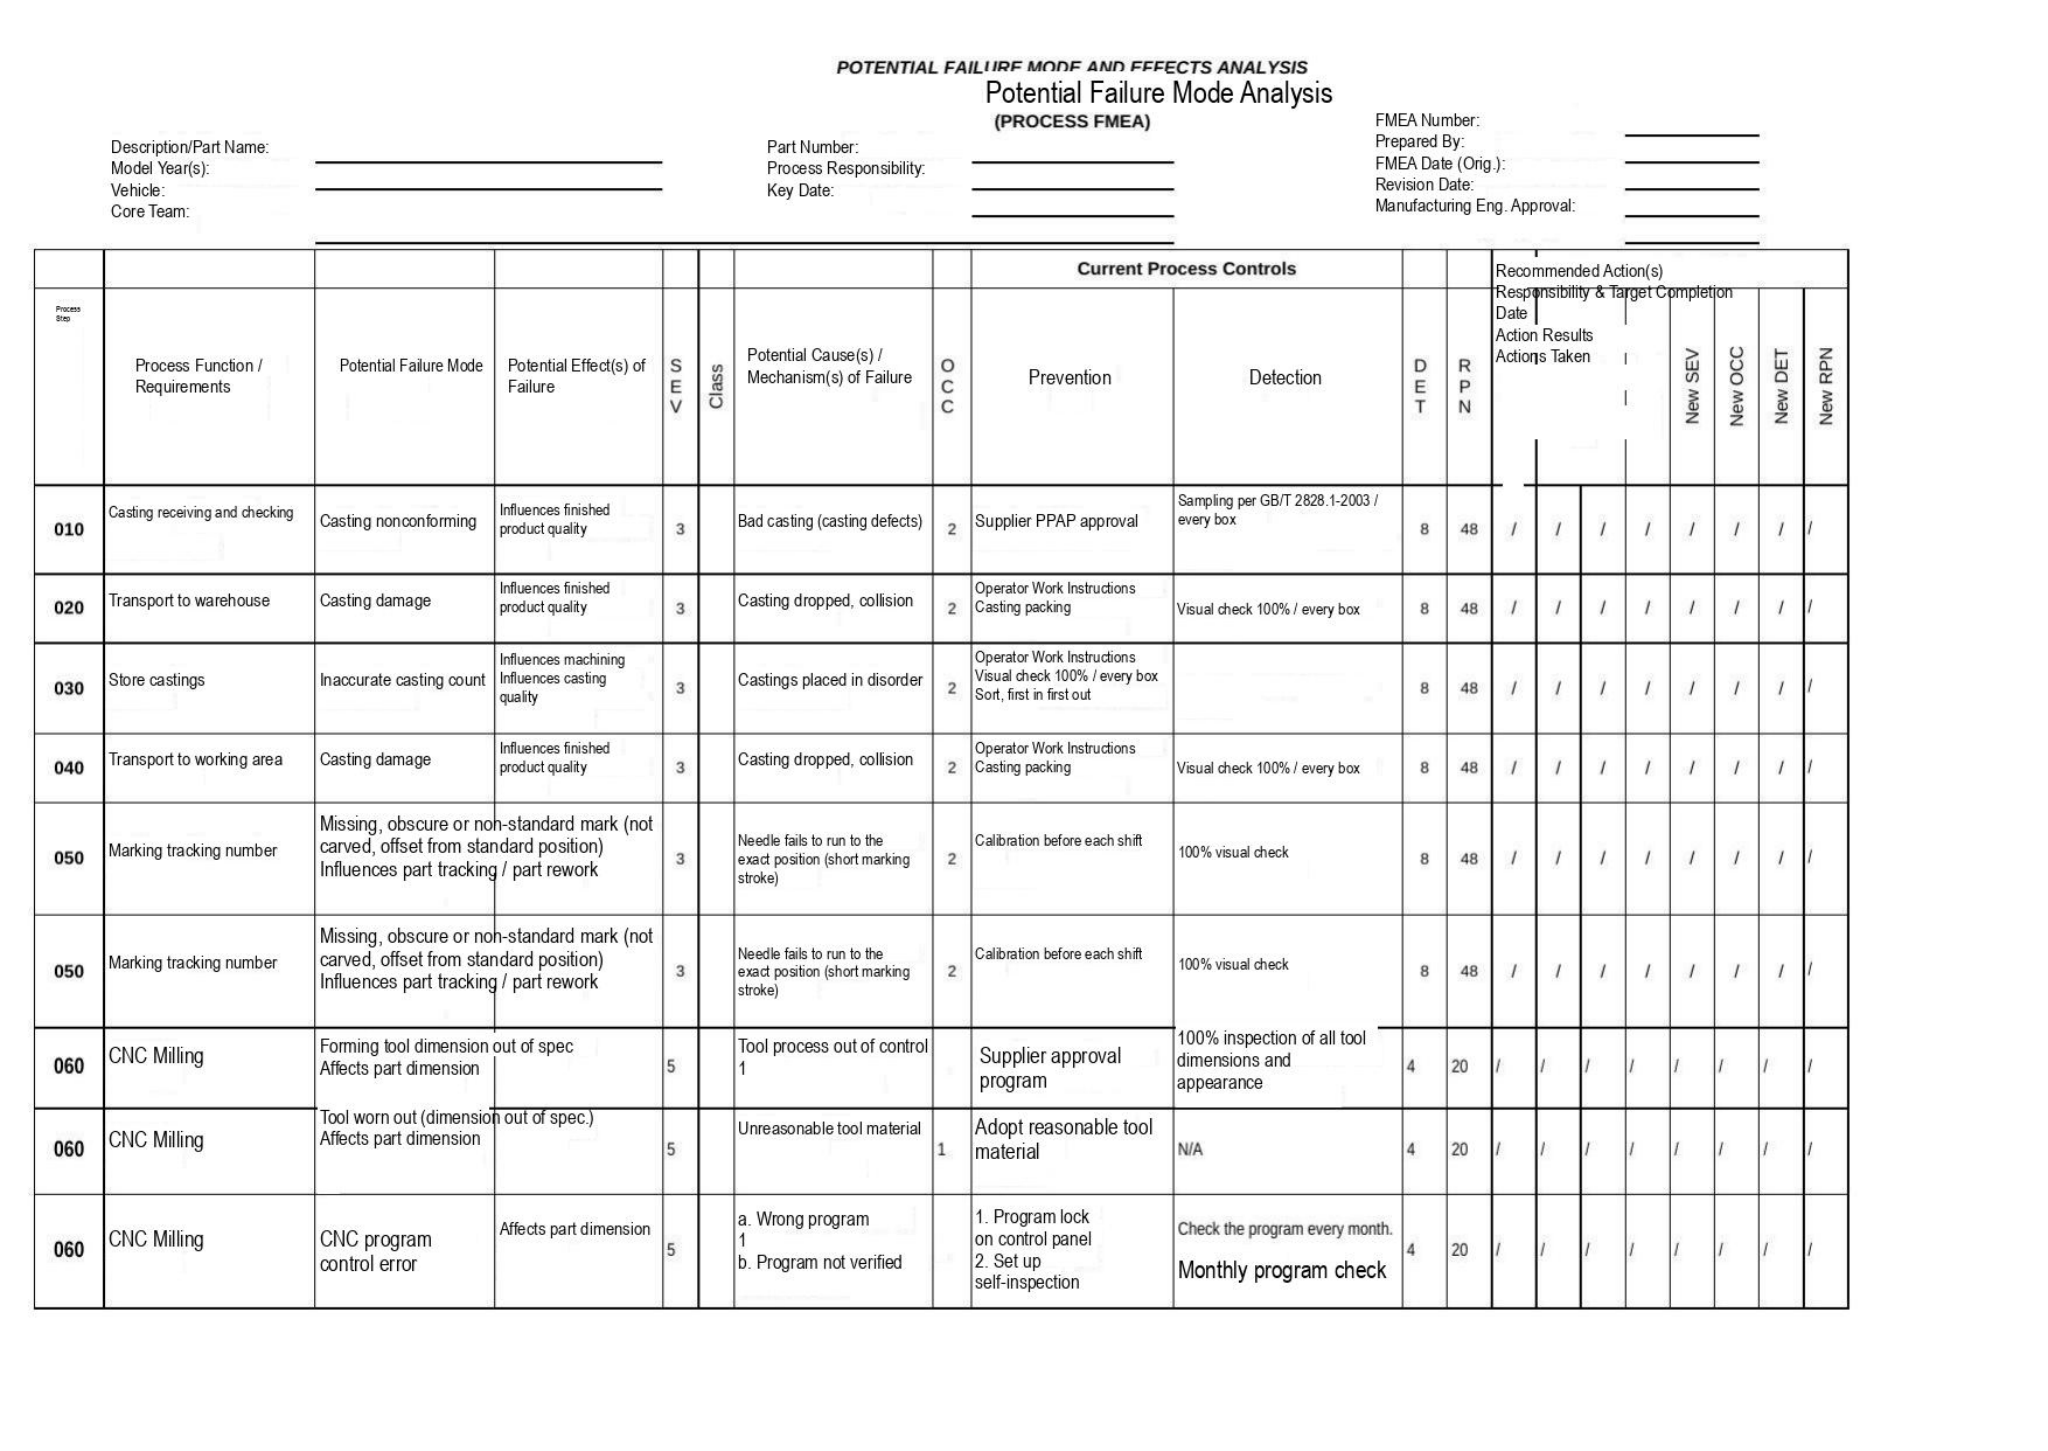POTENTIAL FAILURE MODE AND EFFECTS ANALYSIS
Potential Failure Mode Analysis
(PROCESS FMEA)

Description/Part Name:
Model Year(s):
Vehicle:
Core Team:

Part Number:
Process Responsibility:
Key Date:

FMEA Number:
Prepared By:
FMEA Date (Orig.):
Revision Date:
Manufacturing Eng. Approval:

| Process Step | Process Function / Requirements | Potential Failure Mode | Potential Effect(s) of Failure | SEV | Class | Potential Cause(s) / Mechanism(s) of Failure | OCC | Current Process Controls: Prevention | Current Process Controls: Detection | DET | RPN | Recommended Action(s) Responsibility & Target Completion Date Action Results Actions Taken | | | | New SEV | New OCC | New DET | New RPN |
|---|---|---|---|---|---|---|---|---|---|---|---|---|---|---|---|---|---|---|---|
| 010 | Casting receiving and checking | Casting nonconforming | Influences finished product quality | 3 | | Bad casting (casting defects) | 2 | Supplier PPAP approval | Sampling per GB/T 2828.1-2003 / every box | 8 | 48 | / | / | / | / | / | / | / | / |
| 020 | Transport to warehouse | Casting damage | Influences finished product quality | 3 | | Casting dropped, collision | 2 | Operator Work Instructions Casting packing | Visual check 100% / every box | 8 | 48 | / | / | / | / | / | / | / | / |
| 030 | Store castings | Inaccurate casting count | Influences machining Influences casting quality | 3 | | Castings placed in disorder | 2 | Operator Work Instructions Visual check 100% / every box Sort, first in first out | | 8 | 48 | / | / | / | / | / | / | / | / |
| 040 | Transport to working area | Casting damage | Influences finished product quality | 3 | | Casting dropped, collision | 2 | Operator Work Instructions Casting packing | Visual check 100% / every box | 8 | 48 | / | / | / | / | / | / | / | / |
| 050 | Marking tracking number | Missing, obscure or non-standard mark (not carved, offset from standard position) Influences part tracking / part rework | | 3 | | Needle fails to run to the exact position (short marking stroke) | 2 | Calibration before each shift | 100% visual check | 8 | 48 | / | / | / | / | / | / | / | / |
| 050 | Marking tracking number | Missing, obscure or non-standard mark (not carved, offset from standard position) Influences part tracking / part rework | | 3 | | Needle fails to run to the exact position (short marking stroke) | 2 | Calibration before each shift | 100% visual check | 8 | 48 | / | / | / | / | / | / | / | / |
| 060 | CNC Milling | Forming tool dimension out of spec Affects part dimension | | 5 | | Tool process out of control 1 | | Supplier approval program | 100% inspection of all tool dimensions and appearance | 4 | 20 | / | / | / | / | / | / | / | / |
| 060 | CNC Milling | Tool worn out (dimension out of spec.) Affects part dimension | | 5 | | Unreasonable tool material | 1 | Adopt reasonable tool material | N/A | 4 | 20 | / | / | / | / | / | / | / | / |
| 060 | CNC Milling | CNC program control error | Affects part dimension | 5 | | a. Wrong program 1 b. Program not verified | | 1. Program lock on control panel 2. Set up self-inspection | Check the program every month. Monthly program check | 4 | 20 | / | / | / | / | / | / | / | / |
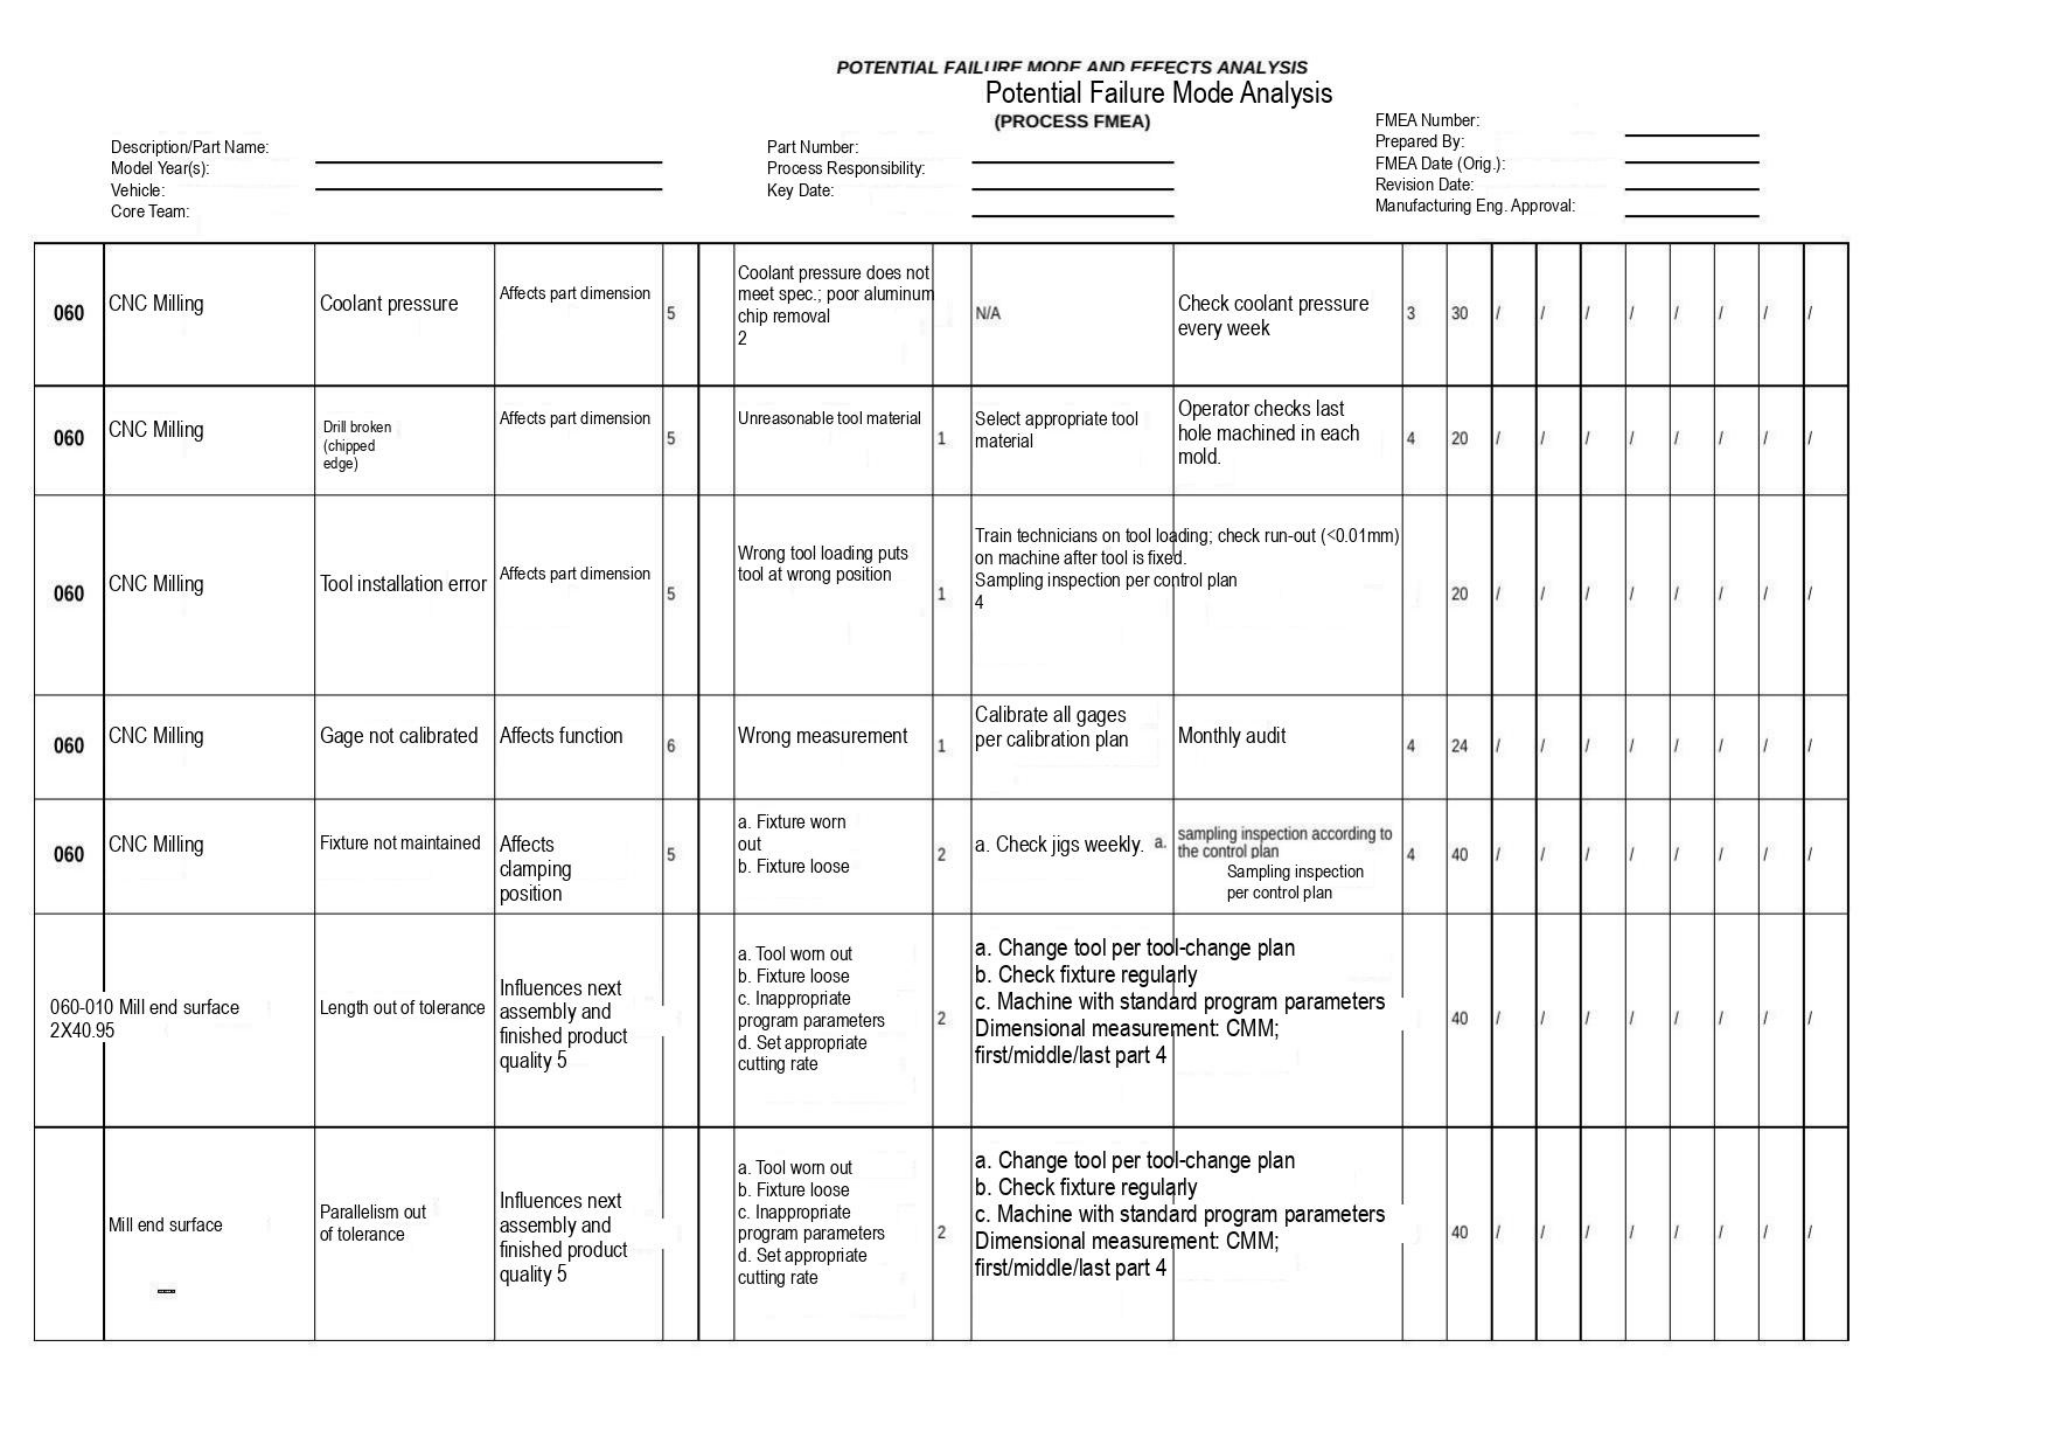POTENTIAL FAILURE MODE AND EFFECTS ANALYSIS
Potential Failure Mode Analysis
(PROCESS FMEA)

Description/Part Name:
Model Year(s):
Vehicle:
Core Team:

Part Number:
Process Responsibility:
Key Date:

FMEA Number:
Prepared By:
FMEA Date (Orig.):
Revision Date:
Manufacturing Eng. Approval:

| | | | | | | | | | | | | | | | | | | | | |
|---|---|---|---|---|---|---|---|---|---|---|---|---|---|---|---|---|---|---|---|---|
| 060 | CNC Milling | Coolant pressure | Affects part dimension | 5 | | Coolant pressure does not meet spec.; poor aluminum chip removal 2 | | N/A | Check coolant pressure every week | 3 | 30 | / | / | / | / | / | / | / | / |
| 060 | CNC Milling | Drill broken (chipped edge) | Affects part dimension | 5 | | Unreasonable tool material | 1 | Select appropriate tool material | Operator checks last hole machined in each mold. | 4 | 20 | / | / | / | / | / | / | / | / |
| 060 | CNC Milling | Tool installation error | Affects part dimension | 5 | | Wrong tool loading puts tool at wrong position | 1 | Train technicians on tool loading; check run-out (<0.01mm) on machine after tool is fixed. Sampling inspection per control plan 4 | | | 20 | / | / | / | / | / | / | / | / |
| 060 | CNC Milling | Gage not calibrated | Affects function | 6 | | Wrong measurement | 1 | Calibrate all gages per calibration plan | Monthly audit | 4 | 24 | / | / | / | / | / | / | / | / |
| 060 | CNC Milling | Fixture not maintained | Affects clamping position | 5 | | a. Fixture worn out b. Fixture loose | 2 | a. Check jigs weekly. | a. sampling inspection according to the control plan Sampling inspection per control plan | 4 | 40 | / | / | / | / | / | / | / | / |
| 060-010 Mill end surface 2X40.95 | | Length out of tolerance | Influences next assembly and finished product quality 5 | | | a. Tool worn out b. Fixture loose c. Inappropriate program parameters d. Set appropriate cutting rate | 2 | a. Change tool per tool-change plan b. Check fixture regularly c. Machine with standard program parameters Dimensional measurement: CMM; first/middle/last part 4 | | | 40 | / | / | / | / | / | / | / | / |
| | Mill end surface | Parallelism out of tolerance | Influences next assembly and finished product quality 5 | | | a. Tool worn out b. Fixture loose c. Inappropriate program parameters d. Set appropriate cutting rate | 2 | a. Change tool per tool-change plan b. Check fixture regularly c. Machine with standard program parameters Dimensional measurement: CMM; first/middle/last part 4 | | | 40 | / | / | / | / | / | / | / | / |
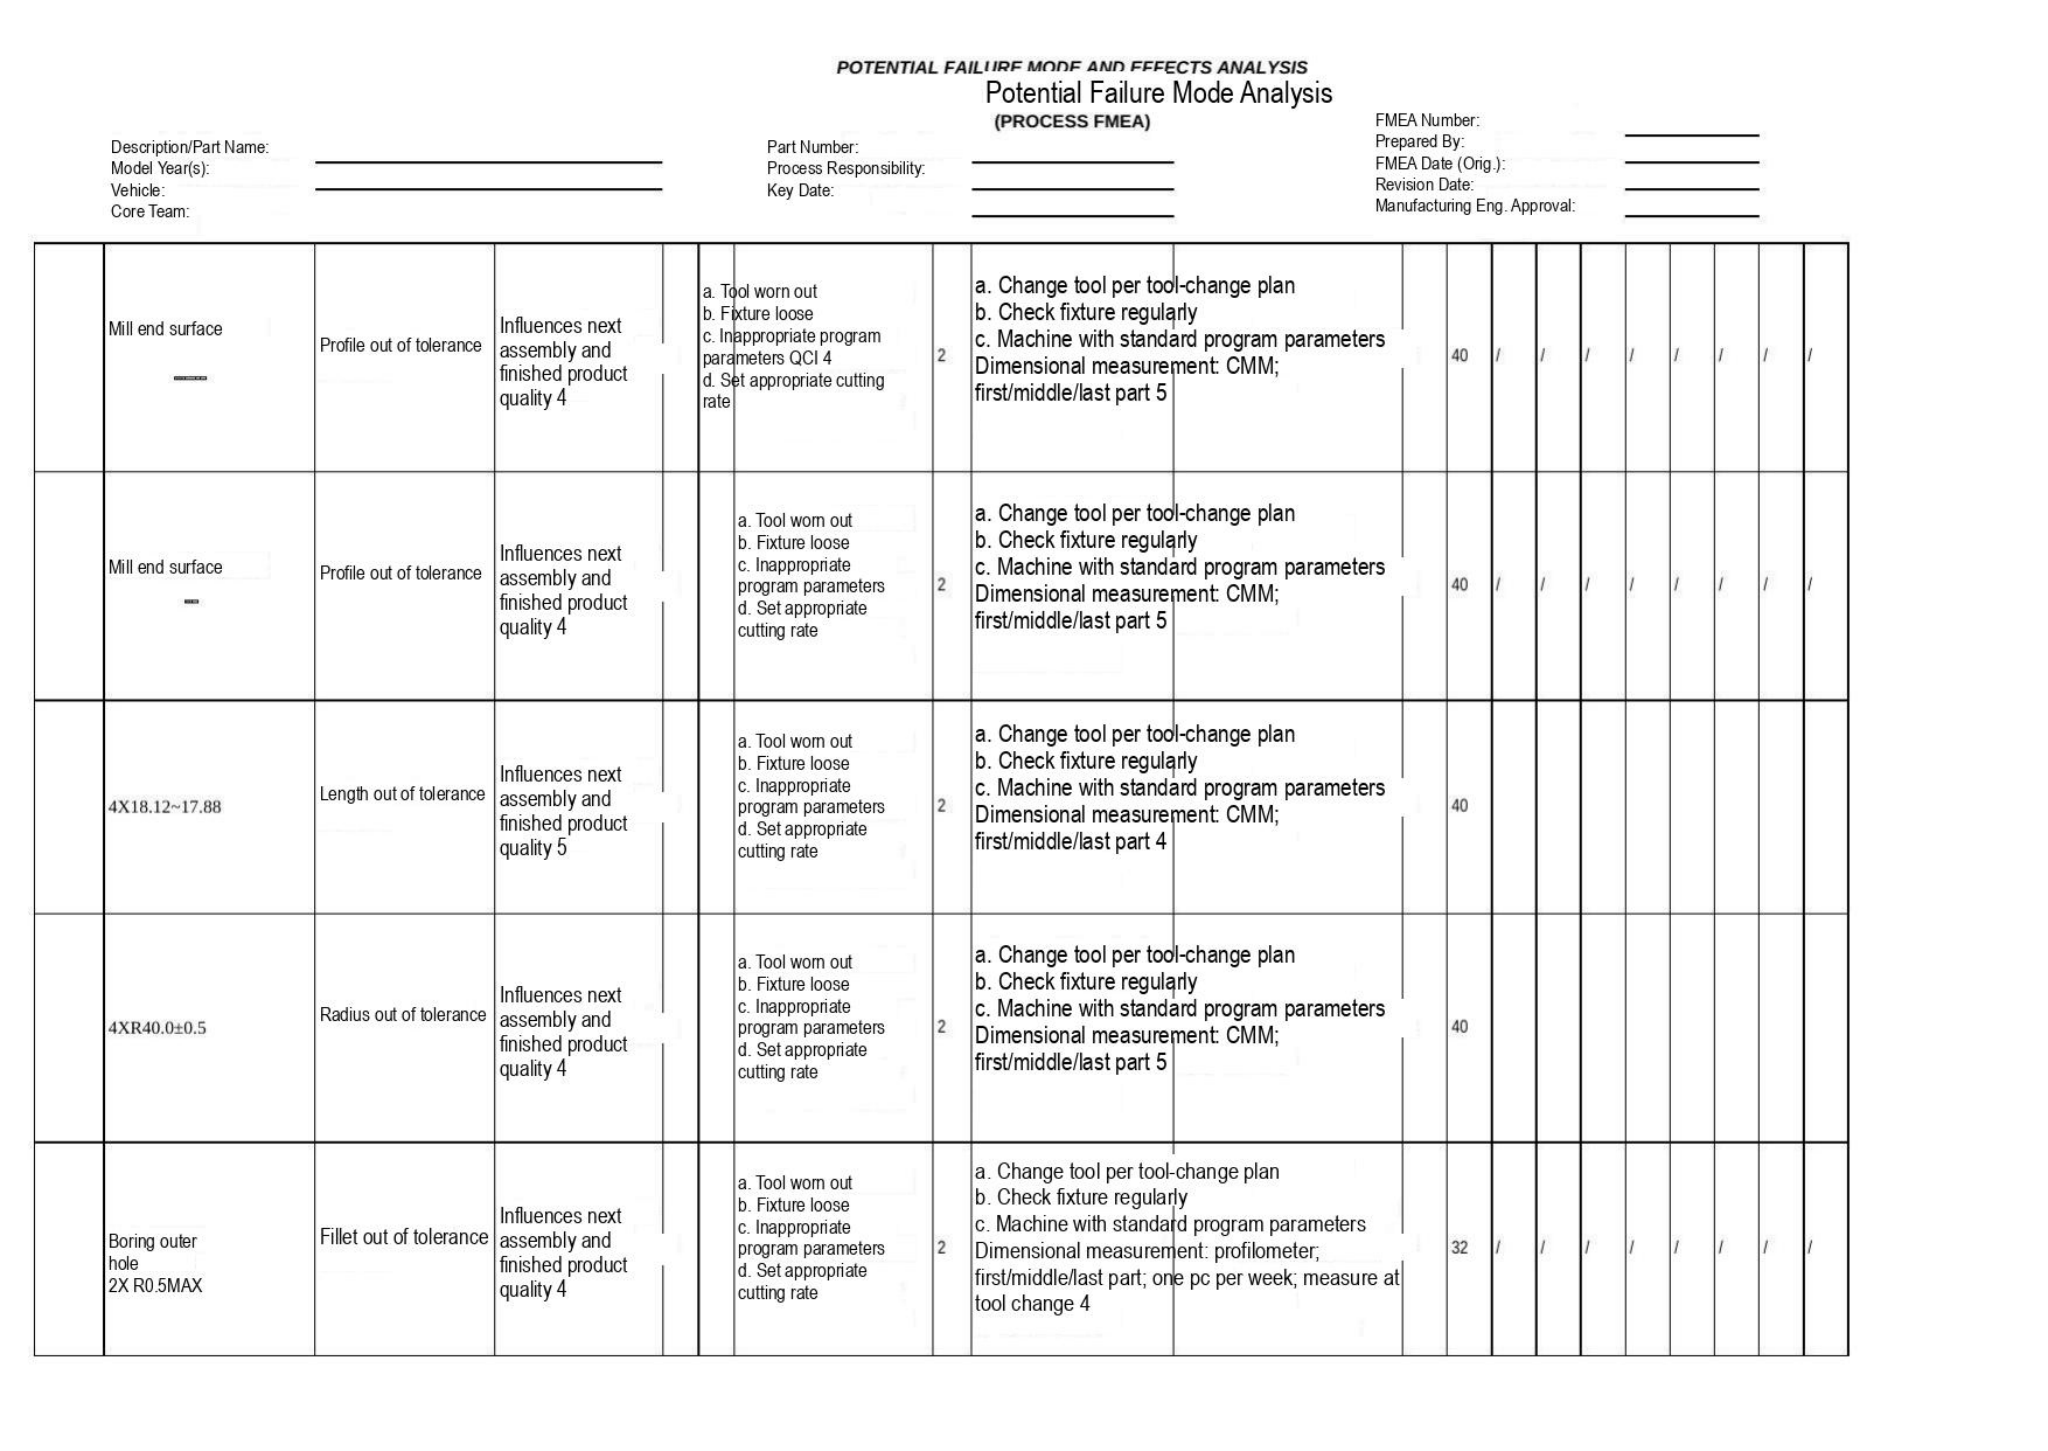POTENTIAL FAILURE MODE AND EFFECTS ANALYSIS

Potential Failure Mode Analysis

(PROCESS FMEA)

Description/Part Name:
Model Year(s):
Vehicle:
Core Team:

Part Number:
Process Responsibility:
Key Date:

FMEA Number:
Prepared By:
FMEA Date (Orig.):
Revision Date:
Manufacturing Eng. Approval:

| | | | | | | | | | | | | | | | | | | | | |
|---|---|---|---|---|---|---|---|---|---|---|---|---|---|---|---|---|---|---|---|---|
| | Mill end surface | Profile out of tolerance | Influences next assembly and finished product quality 4 | | a. Tool worn out<br>b. Fixture loose<br>c. Inappropriate program parameters QCI 4<br>d. Set appropriate cutting rate | | 2 | a. Change tool per tool-change plan<br>b. Check fixture regularly<br>c. Machine with standard program parameters<br>Dimensional measurement: CMM;<br>first/middle/last part 5 | | | 40 | / | / | / | / | / | / | / | / | |
| | Mill end surface | Profile out of tolerance | Influences next assembly and finished product quality 4 | | | a. Tool worn out<br>b. Fixture loose<br>c. Inappropriate program parameters<br>d. Set appropriate cutting rate | 2 | a. Change tool per tool-change plan<br>b. Check fixture regularly<br>c. Machine with standard program parameters<br>Dimensional measurement: CMM;<br>first/middle/last part 5 | | | 40 | / | / | / | / | / | / | / | / | |
| | 4X18.12~17.88 | Length out of tolerance | Influences next assembly and finished product quality 5 | | | a. Tool worn out<br>b. Fixture loose<br>c. Inappropriate program parameters<br>d. Set appropriate cutting rate | 2 | a. Change tool per tool-change plan<br>b. Check fixture regularly<br>c. Machine with standard program parameters<br>Dimensional measurement: CMM;<br>first/middle/last part 4 | | | 40 | | | | | | | | | |
| | 4XR40.0±0.5 | Radius out of tolerance | Influences next assembly and finished product quality 4 | | | a. Tool worn out<br>b. Fixture loose<br>c. Inappropriate program parameters<br>d. Set appropriate cutting rate | 2 | a. Change tool per tool-change plan<br>b. Check fixture regularly<br>c. Machine with standard program parameters<br>Dimensional measurement: CMM;<br>first/middle/last part 5 | | | 40 | | | | | | | | | |
| | Boring outer hole<br>2X R0.5MAX | Fillet out of tolerance | Influences next assembly and finished product quality 4 | | | a. Tool worn out<br>b. Fixture loose<br>c. Inappropriate program parameters<br>d. Set appropriate cutting rate | 2 | a. Change tool per tool-change plan<br>b. Check fixture regularly<br>c. Machine with standard program parameters<br>Dimensional measurement: profilometer;<br>first/middle/last part; one pc per week; measure at tool change 4 | | | 32 | / | / | / | / | / | / | / | / | |
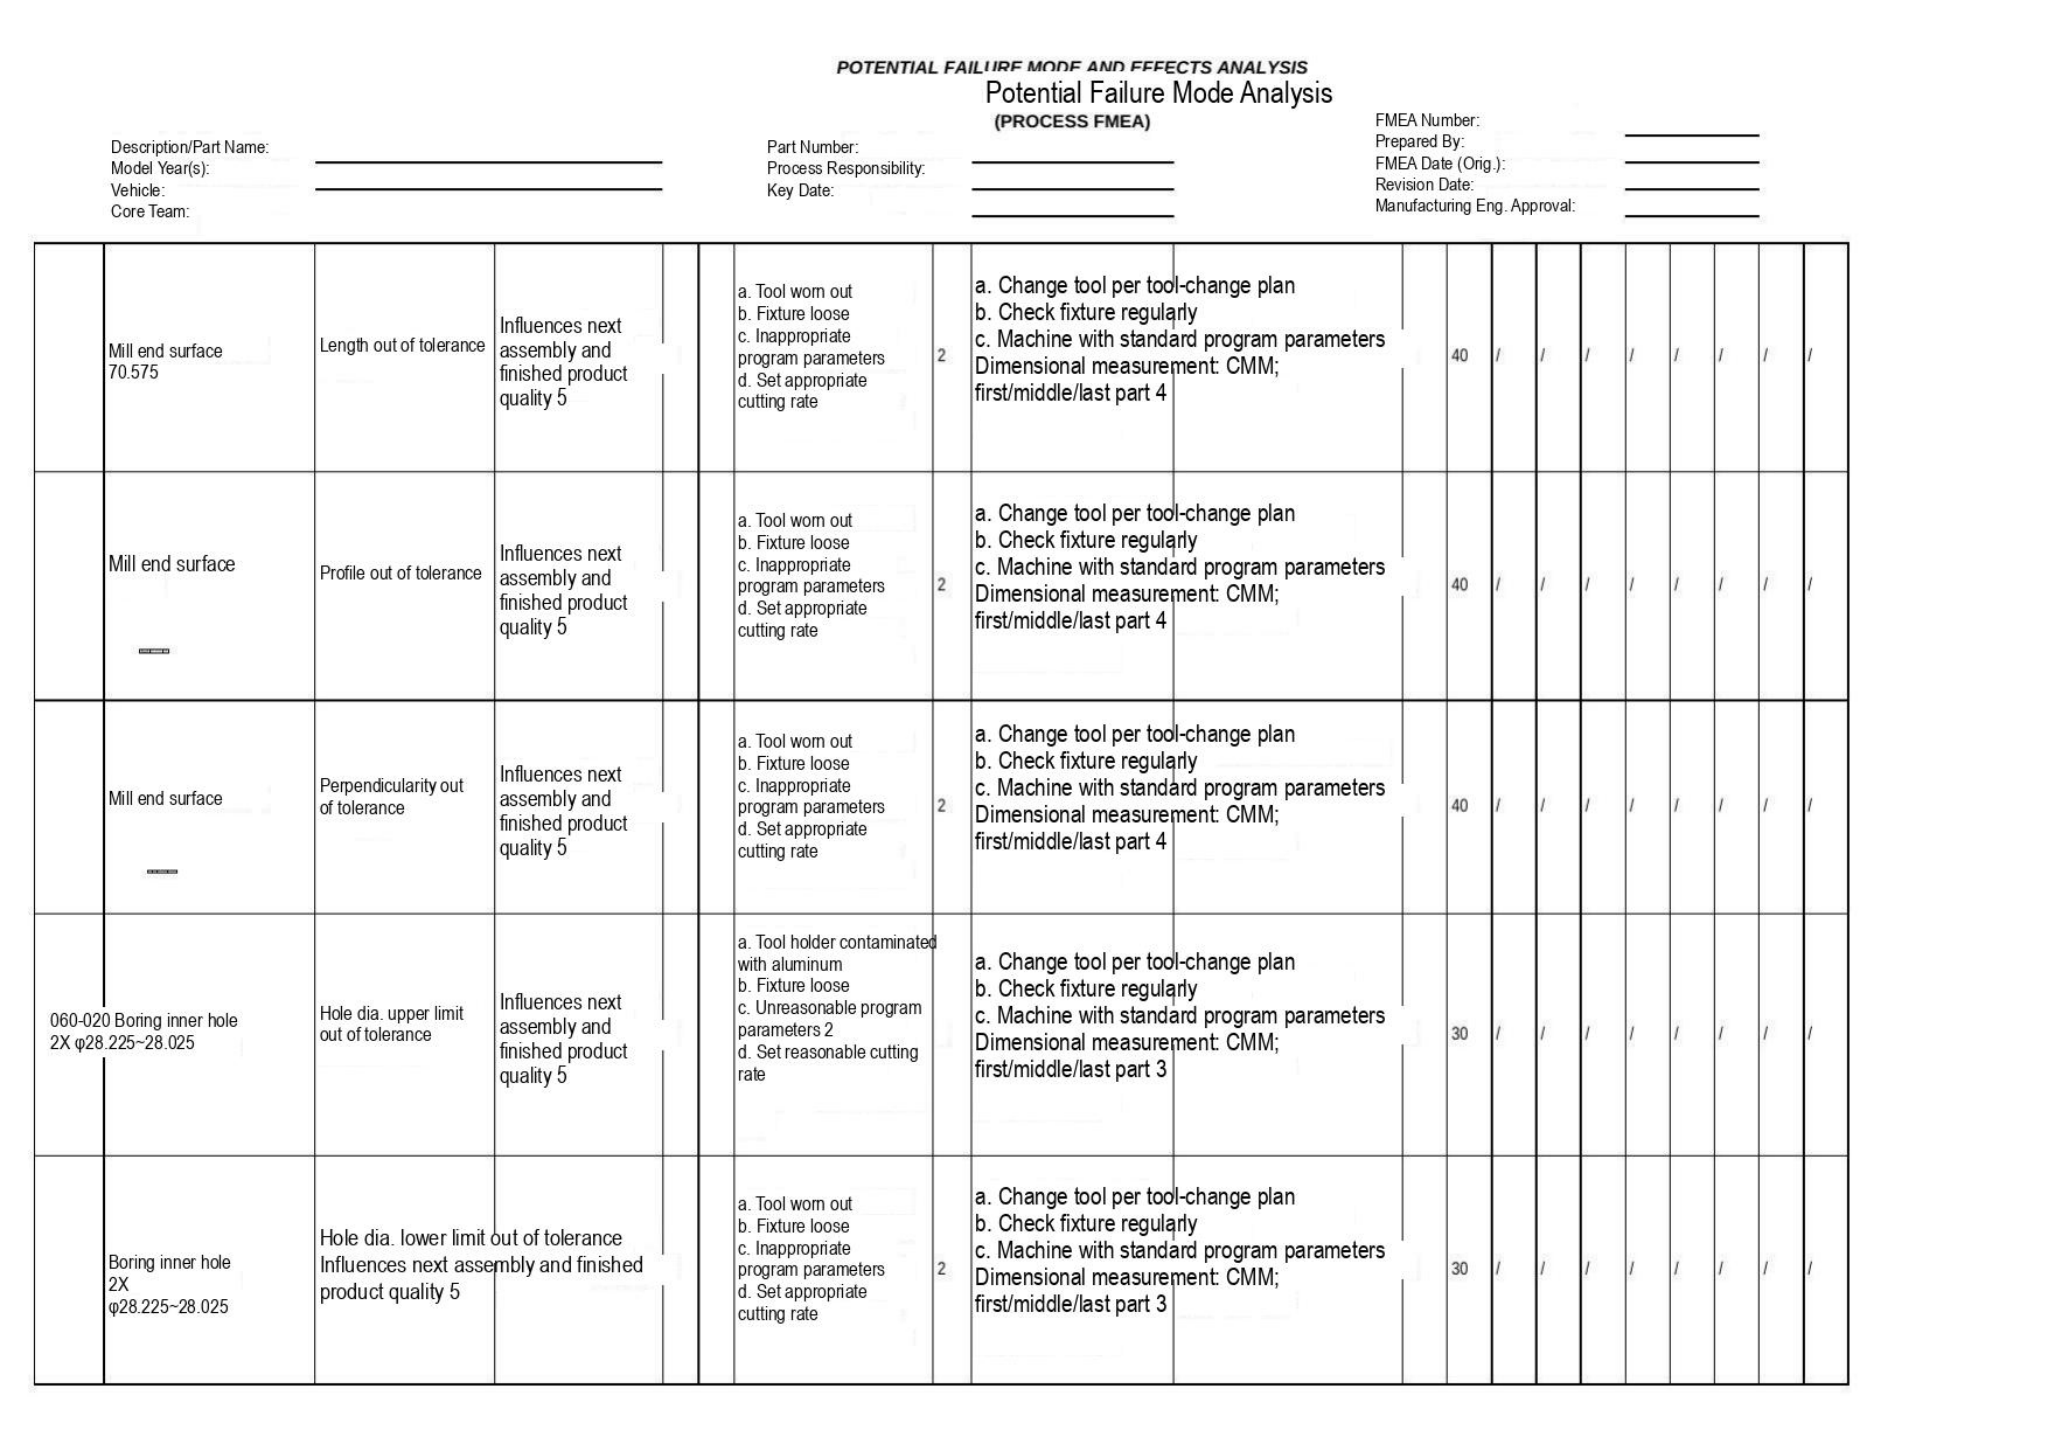POTENTIAL FAILURE MODE AND EFFECTS ANALYSIS
Potential Failure Mode Analysis
(PROCESS FMEA)

Description/Part Name:
Model Year(s):
Vehicle:
Core Team:

Part Number:
Process Responsibility:
Key Date:

FMEA Number:
Prepared By:
FMEA Date (Orig.):
Revision Date:
Manufacturing Eng. Approval:

| | | | | | | | | | | | | | | | | | | | |
|---|---|---|---|---|---|---|---|---|---|---|---|---|---|---|---|---|---|---|---|
| | Mill end surface 70.575 | Length out of tolerance | Influences next assembly and finished product quality 5 | | | a. Tool worn out b. Fixture loose c. Inappropriate program parameters d. Set appropriate cutting rate | 2 | a. Change tool per tool-change plan b. Check fixture regularly c. Machine with standard program parameters Dimensional measurement: CMM; first/middle/last part 4 | | | 40 | / | / | / | / | / | / | / | / |
| | Mill end surface | Profile out of tolerance | Influences next assembly and finished product quality 5 | | | a. Tool worn out b. Fixture loose c. Inappropriate program parameters d. Set appropriate cutting rate | 2 | a. Change tool per tool-change plan b. Check fixture regularly c. Machine with standard program parameters Dimensional measurement: CMM; first/middle/last part 4 | | | 40 | / | / | / | / | / | / | / | / |
| | Mill end surface | Perpendicularity out of tolerance | Influences next assembly and finished product quality 5 | | | a. Tool worn out b. Fixture loose c. Inappropriate program parameters d. Set appropriate cutting rate | 2 | a. Change tool per tool-change plan b. Check fixture regularly c. Machine with standard program parameters Dimensional measurement: CMM; first/middle/last part 4 | | | 40 | / | / | / | / | / | / | / | / |
| 060-020 | Boring inner hole 2X φ28.225~28.025 | Hole dia. upper limit out of tolerance | Influences next assembly and finished product quality 5 | | | a. Tool holder contaminated with aluminum b. Fixture loose c. Unreasonable program parameters 2 d. Set reasonable cutting rate | | a. Change tool per tool-change plan b. Check fixture regularly c. Machine with standard program parameters Dimensional measurement: CMM; first/middle/last part 3 | | | 30 | / | / | / | / | / | / | / | / |
| | Boring inner hole 2X φ28.225~28.025 | Hole dia. lower limit out of tolerance Influences next assembly and finished product quality 5 | | | | a. Tool worn out b. Fixture loose c. Inappropriate program parameters d. Set appropriate cutting rate | 2 | a. Change tool per tool-change plan b. Check fixture regularly c. Machine with standard program parameters Dimensional measurement: CMM; first/middle/last part 3 | | | 30 | / | / | / | / | / | / | / | / |
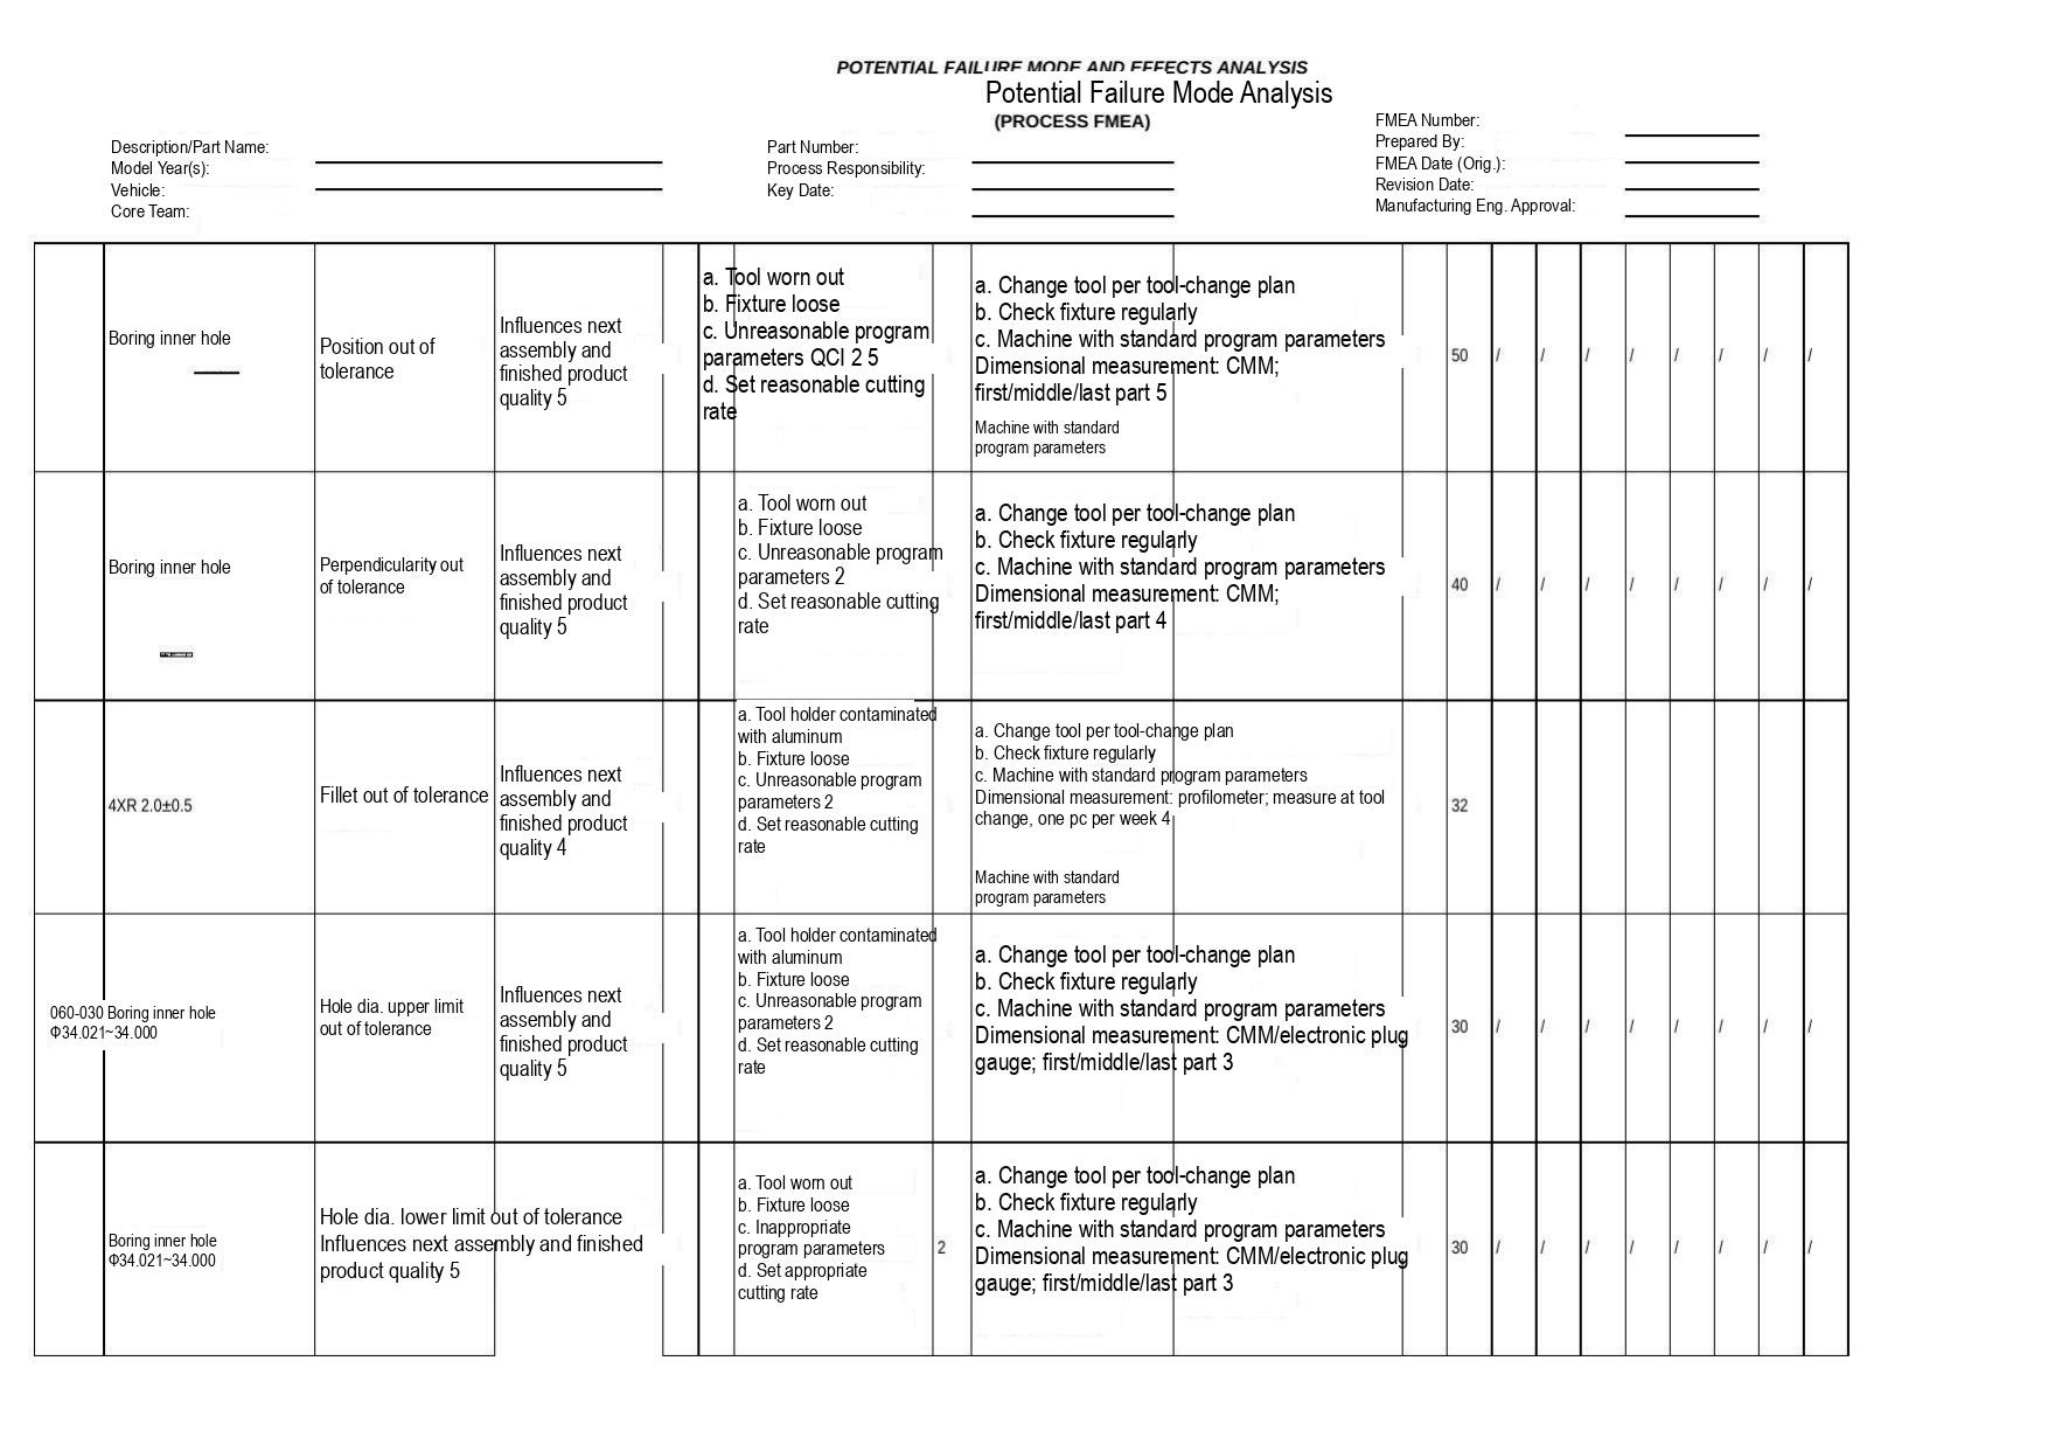POTENTIAL FAILURE MODE AND EFFECTS ANALYSIS
Potential Failure Mode Analysis
(PROCESS FMEA)

Description/Part Name:
Model Year(s):
Vehicle:
Core Team:

Part Number:
Process Responsibility:
Key Date:

FMEA Number:
Prepared By:
FMEA Date (Orig.):
Revision Date:
Manufacturing Eng. Approval:

| | | | | | | | | | | | | | | | | | | |
|---|---|---|---|---|---|---|---|---|---|---|---|---|---|---|---|---|---|---|
| | Boring inner hole | Position out of tolerance | Influences next assembly and finished product quality 5 | | a. Tool worn out<br>b. Fixture loose<br>c. Unreasonable program parameters QCI 2 5<br>d. Set reasonable cutting rate | | | a. Change tool per tool-change plan<br>b. Check fixture regularly<br>c. Machine with standard program parameters<br>Dimensional measurement: CMM; first/middle/last part 5<br>Machine with standard program parameters | | 50 | / | / | / | / | / | / | / | / |
| | Boring inner hole | Perpendicularity out of tolerance | Influences next assembly and finished product quality 5 | | | a. Tool worn out<br>b. Fixture loose<br>c. Unreasonable program parameters 2<br>d. Set reasonable cutting rate | | a. Change tool per tool-change plan<br>b. Check fixture regularly<br>c. Machine with standard program parameters<br>Dimensional measurement: CMM; first/middle/last part 4 | | 40 | / | / | / | / | / | / | / | / |
| | 4XR 2.0±0.5 | Fillet out of tolerance | Influences next assembly and finished product quality 4 | | | a. Tool holder contaminated with aluminum<br>b. Fixture loose<br>c. Unreasonable program parameters 2<br>d. Set reasonable cutting rate | | a. Change tool per tool-change plan<br>b. Check fixture regularly<br>c. Machine with standard program parameters<br>Dimensional measurement: profilometer; measure at tool change, one pc per week 4<br>Machine with standard program parameters | | 32 | | | | | | | | |
| 060-030 | Boring inner hole Φ34.021~34.000 | Hole dia. upper limit out of tolerance | Influences next assembly and finished product quality 5 | | | a. Tool holder contaminated with aluminum<br>b. Fixture loose<br>c. Unreasonable program parameters 2<br>d. Set reasonable cutting rate | | a. Change tool per tool-change plan<br>b. Check fixture regularly<br>c. Machine with standard program parameters<br>Dimensional measurement: CMM/electronic plug gauge; first/middle/last part 3 | | 30 | / | / | / | / | / | / | / | / |
| | Boring inner hole Φ34.021~34.000 | Hole dia. lower limit out of tolerance Influences next assembly and finished product quality 5 | | | | a. Tool worn out<br>b. Fixture loose<br>c. Inappropriate program parameters<br>d. Set appropriate cutting rate | 2 | a. Change tool per tool-change plan<br>b. Check fixture regularly<br>c. Machine with standard program parameters<br>Dimensional measurement: CMM/electronic plug gauge; first/middle/last part 3 | | 30 | / | / | / | / | / | / | / | / |
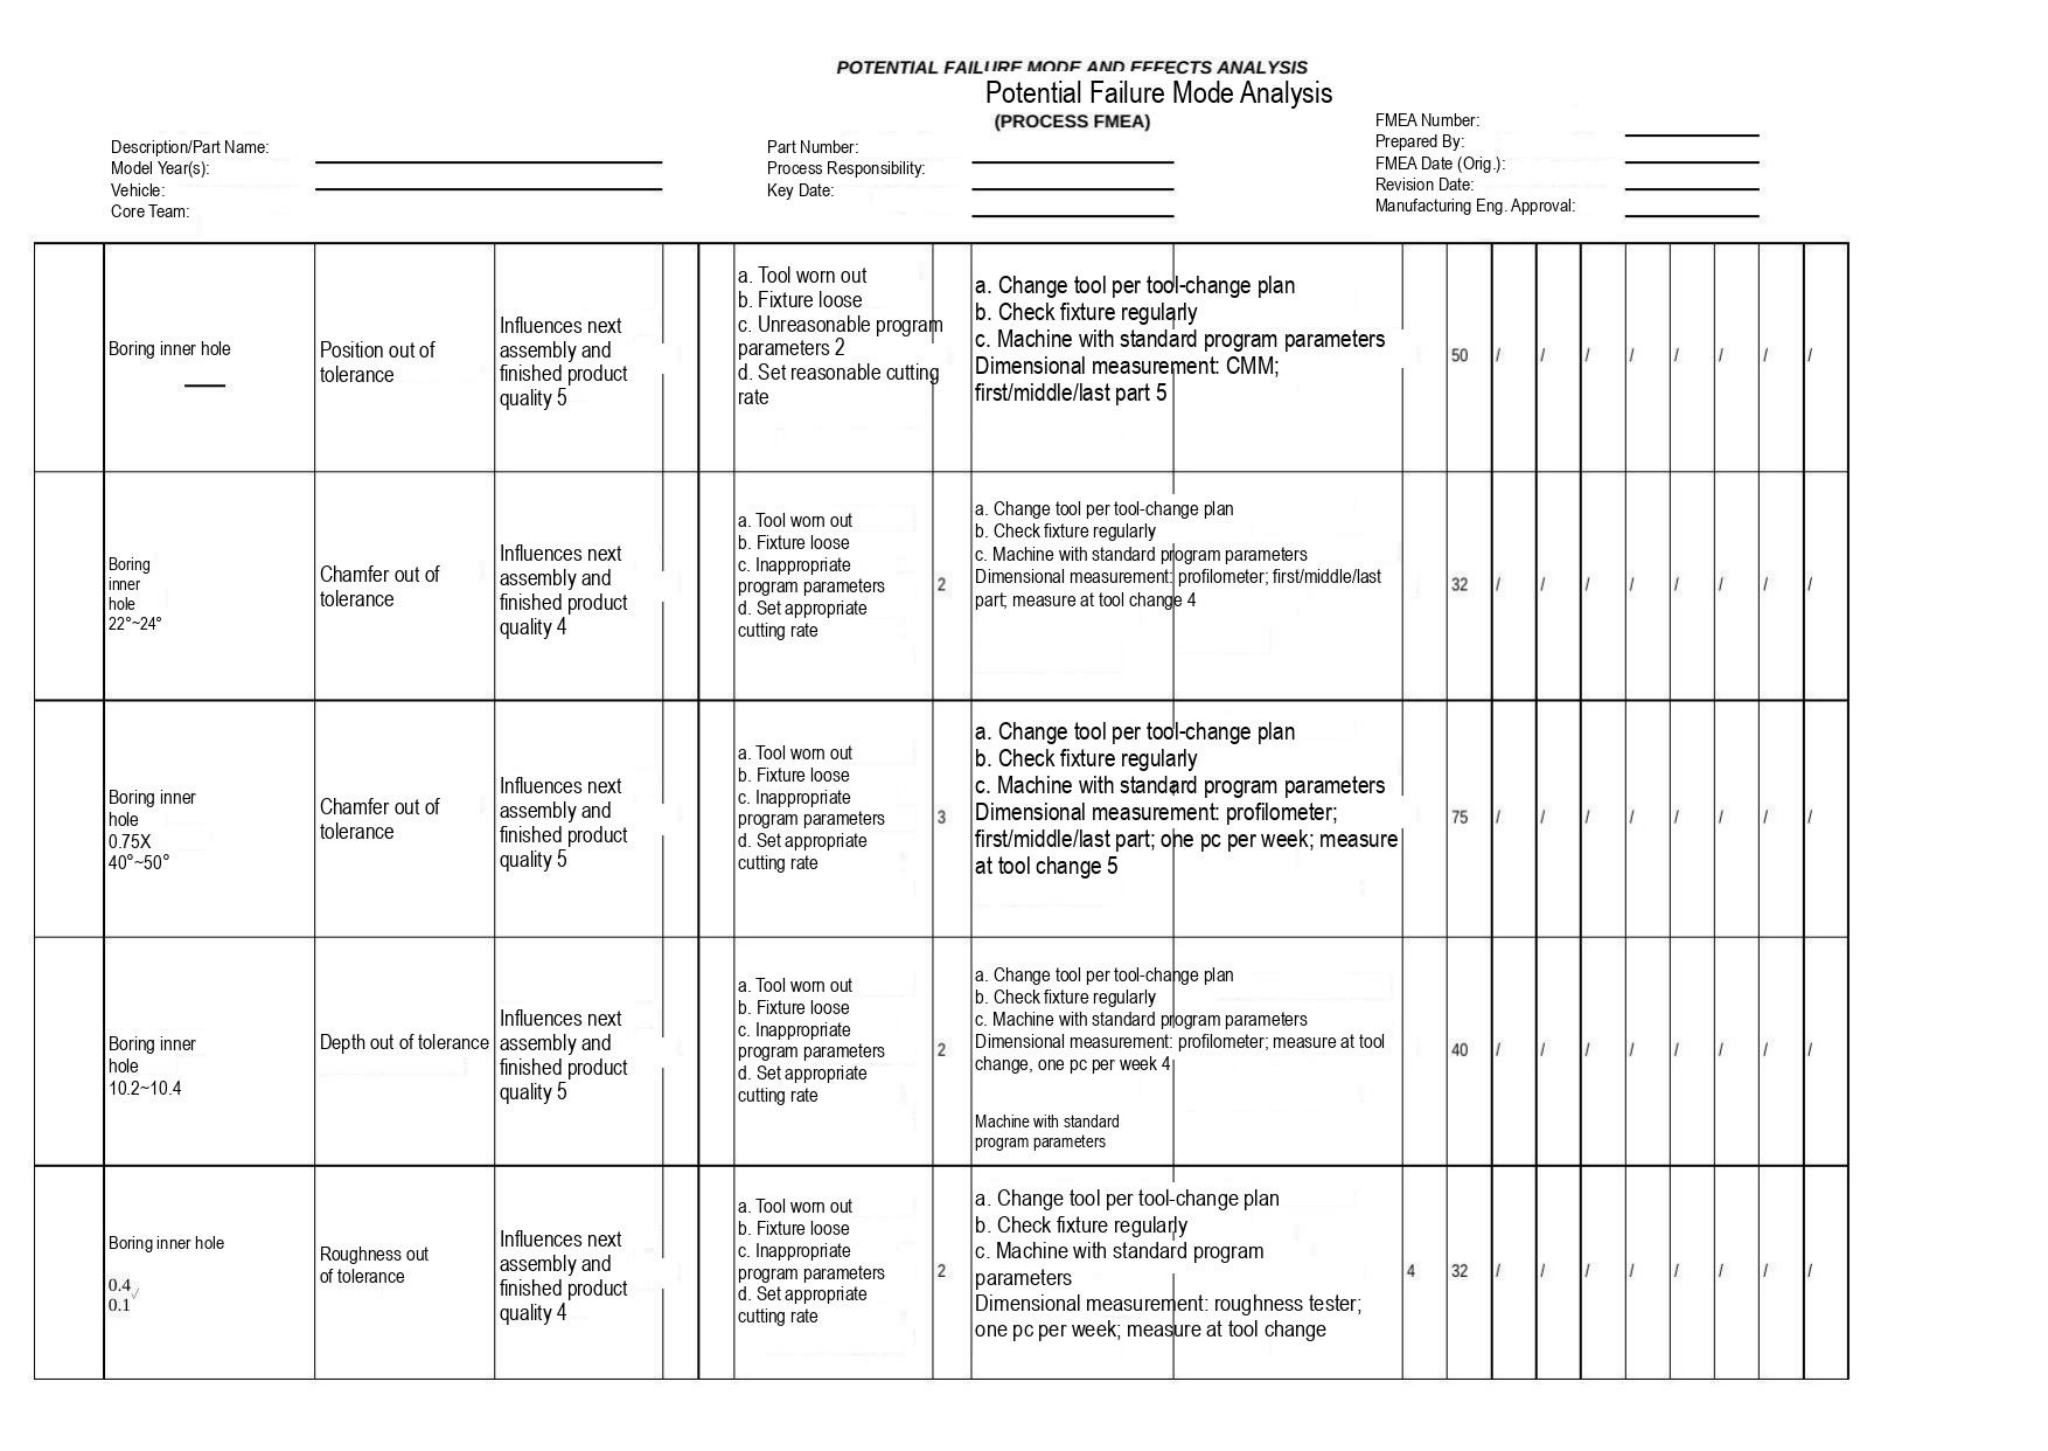**POTENTIAL FAILURE MODE AND EFFECTS ANALYSIS**

Potential Failure Mode Analysis

**(PROCESS FMEA)**

Description/Part Name:
Model Year(s):
Vehicle:
Core Team:

Part Number:
Process Responsibility:
Key Date:

FMEA Number:
Prepared By:
FMEA Date (Orig.):
Revision Date:
Manufacturing Eng. Approval:

| | | | | | | | | | | | | | | | | | | |
|---|---|---|---|---|---|---|---|---|---|---|---|---|---|---|---|---|---|---|
| | Boring inner hole | Position out of tolerance | Influences next assembly and finished product quality 5 | | | a. Tool worn out<br>b. Fixture loose<br>c. Unreasonable program parameters 2<br>d. Set reasonable cutting rate | | a. Change tool per tool-change plan<br>b. Check fixture regularly<br>c. Machine with standard program parameters<br>Dimensional measurement: CMM; first/middle/last part 5 | | 50 | / | / | / | / | / | / | / | / |
| | Boring inner hole 22°~24° | Chamfer out of tolerance | Influences next assembly and finished product quality 4 | | | a. Tool worn out<br>b. Fixture loose<br>c. Inappropriate program parameters<br>d. Set appropriate cutting rate | 2 | a. Change tool per tool-change plan<br>b. Check fixture regularly<br>c. Machine with standard program parameters<br>Dimensional measurement: profilometer; first/middle/last part; measure at tool change 4 | | 32 | / | / | / | / | / | / | / | / |
| | Boring inner hole 0.75X 40°~50° | Chamfer out of tolerance | Influences next assembly and finished product quality 5 | | | a. Tool worn out<br>b. Fixture loose<br>c. Inappropriate program parameters<br>d. Set appropriate cutting rate | 3 | a. Change tool per tool-change plan<br>b. Check fixture regularly<br>c. Machine with standard program parameters<br>Dimensional measurement: profilometer; first/middle/last part; one pc per week; measure at tool change 5 | | 75 | / | / | / | / | / | / | / | / |
| | Boring inner hole 10.2~10.4 | Depth out of tolerance | Influences next assembly and finished product quality 5 | | | a. Tool worn out<br>b. Fixture loose<br>c. Inappropriate program parameters<br>d. Set appropriate cutting rate | 2 | a. Change tool per tool-change plan<br>b. Check fixture regularly<br>c. Machine with standard program parameters<br>Dimensional measurement: profilometer; measure at tool change, one pc per week 4<br>Machine with standard program parameters | | 40 | / | / | / | / | / | / | / | / |
| | Boring inner hole 0.4 0.1 | Roughness out of tolerance | Influences next assembly and finished product quality 4 | | | a. Tool worn out<br>b. Fixture loose<br>c. Inappropriate program parameters<br>d. Set appropriate cutting rate | 2 | a. Change tool per tool-change plan<br>b. Check fixture regularly<br>c. Machine with standard program parameters<br>Dimensional measurement: roughness tester; one pc per week; measure at tool change | 4 | 32 | / | / | / | / | / | / | / | / |